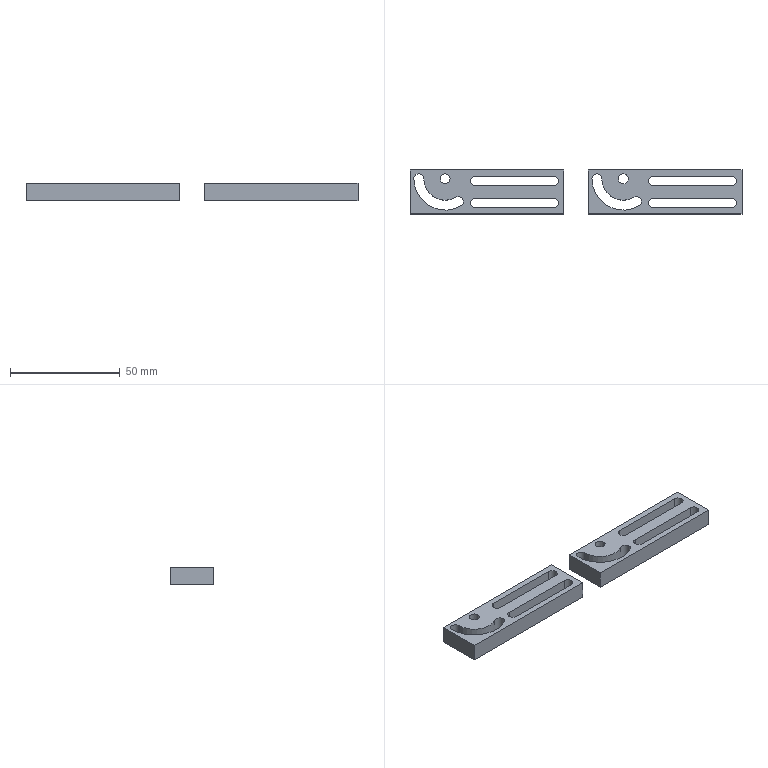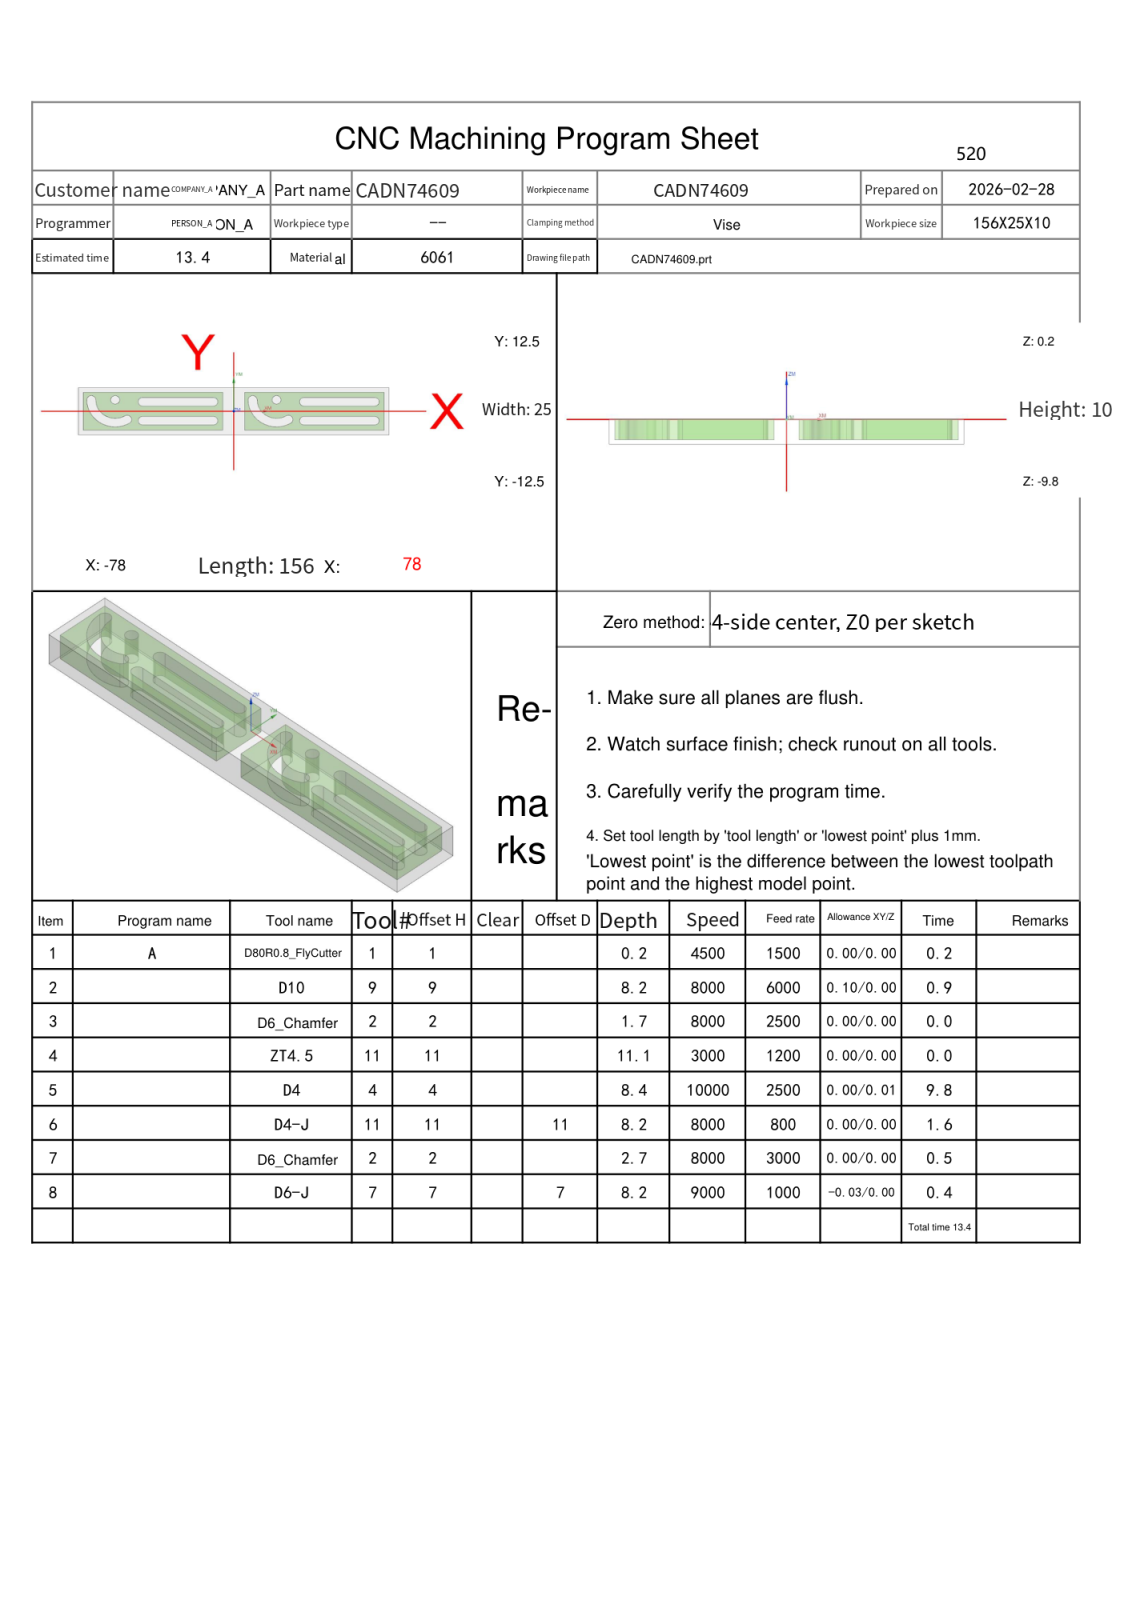NC program | NX | posted by the shop | part box 151 x 20 x 8 mm
Lines 276 to 1289 of 3746:
N5 T04 M06
(D4  D=4. R=0. H=04 ce=0.10 di=0.10)
G00 G90 G54 X-28. Y4.85 M03 S10000
G43 H04 Z50.
M08
Z.5
G01 X-10.25 Z.439 F1200.
G03 X-10.1 Y5. Z.438 I0.0 J.15
X-10.25 Y5.15 Z.437 I-.15 J0.0
G01 X-45.75 Z.314
G03 X-45.9 Y5. Z.314 I0.0 J-.15
X-45.75 Y4.85 Z.313 I.15 J0.0
G01 X-10.25 Z.19
G03 X-10.1 Y5. Z.189 I0.0 J.15
X-10.25 Y5.15 Z.188 I-.15 J0.0
G01 X-45.75 Z.066
G03 X-45.9 Y5. Z.065 I0.0 J-.15
X-45.75 Y4.85 Z.064 I.15 J0.0
G01 X-10.25 Z-.058
G03 X-10.1 Y5. Z-.059 I0.0 J.15
X-10.25 Y5.15 Z-.06 I-.15 J0.0
G01 X-45.75 Z-.183
G03 X-45.9 Y5. Z-.184 I0.0 J-.15
X-45.75 Y4.85 Z-.184 I.15 J0.0
G01 X-10.25 Z-.307
G03 X-10.1 Y5. Z-.308 I0.0 J.15
X-10.25 Y5.15 Z-.309 I-.15 J0.0
G01 X-45.75 Z-.431
G03 X-45.9 Y5. Z-.432 I0.0 J-.15
X-45.75 Y4.85 Z-.433 I.15 J0.0
G01 X-10.25 Z-.556
G03 X-10.1 Y5. Z-.556 I0.0 J.15
X-10.25 Y5.15 Z-.557 I-.15 J0.0
G01 X-45.75 Z-.68
G03 X-45.9 Y5. Z-.681 I0.0 J-.15
X-45.75 Y4.85 Z-.682 I.15 J0.0
G01 X-10.25 Z-.804
G03 X-10.1 Y5. Z-.805 I0.0 J.15
X-10.25 Y5.15 Z-.806 I-.15 J0.0
G01 X-45.75 Z-.928
G03 X-45.9 Y5. Z-.929 I0.0 J-.15
X-45.75 Y4.85 Z-.93 I.15 J0.0
G01 X-10.25 Z-1.053
G03 X-10.1 Y5. Z-1.054 I0.0 J.15
X-10.25 Y5.15 Z-1.054 I-.15 J0.0
G01 X-45.75 Z-1.177
G03 X-45.9 Y5. Z-1.178 I0.0 J-.15
X-45.75 Y4.85 Z-1.179 I.15 J0.0
G01 X-10.25 Z-1.301
G03 X-10.1 Y5. Z-1.302 I0.0 J.15
X-10.25 Y5.15 Z-1.303 I-.15 J0.0
G01 X-45.75 Z-1.426
G03 X-45.9 Y5. Z-1.426 I0.0 J-.15
X-45.75 Y4.85 Z-1.427 I.15 J0.0
G01 X-10.25 Z-1.55
G03 X-10.1 Y5. Z-1.551 I0.0 J.15
X-10.25 Y5.15 Z-1.552 I-.15 J0.0
G01 X-45.75 Z-1.674
G03 X-45.9 Y5. Z-1.675 I0.0 J-.15
X-45.75 Y4.85 Z-1.676 I.15 J0.0
G01 X-10.25 Z-1.798
G03 X-10.1 Y5. Z-1.799 I0.0 J.15
X-10.25 Y5.15 Z-1.8 I-.15 J0.0
G01 X-45.75 Z-1.923
G03 X-45.9 Y5. Z-1.924 I0.0 J-.15
X-45.75 Y4.85 Z-1.924 I.15 J0.0
G01 X-10.25 Z-2.047
G03 X-10.1 Y5. Z-2.048 I0.0 J.15
X-10.25 Y5.15 Z-2.049 I-.15 J0.0
G01 X-45.75 Z-2.171
G03 X-45.9 Y5. Z-2.172 I0.0 J-.15
X-45.75 Y4.85 Z-2.173 I.15 J0.0
G01 X-10.25 Z-2.296
G03 X-10.1 Y5. Z-2.296 I0.0 J.15
X-10.25 Y5.15 Z-2.297 I-.15 J0.0
G01 X-45.75 Z-2.42
G03 X-45.9 Y5. Z-2.421 I0.0 J-.15
X-45.75 Y4.85 Z-2.422 I.15 J0.0
G01 X-10.25 Z-2.544
G03 X-10.1 Y5. Z-2.545 I0.0 J.15
X-10.25 Y5.15 Z-2.546 I-.15 J0.0
G01 X-45.75 Z-2.668
G03 X-45.9 Y5. Z-2.669 I0.0 J-.15
X-45.75 Y4.85 Z-2.67 I.15 J0.0
G01 X-10.25 Z-2.793
G03 X-10.1 Y5. Z-2.794 I0.0 J.15
X-10.25 Y5.15 Z-2.794 I-.15 J0.0
G01 X-45.75 Z-2.917
G03 X-45.9 Y5. Z-2.918 I0.0 J-.15
X-45.75 Y4.85 Z-2.919 I.15 J0.0
G01 X-10.25 Z-3.041
G03 X-10.1 Y5. Z-3.042 I0.0 J.15
X-10.25 Y5.15 Z-3.043 I-.15 J0.0
G01 X-45.75 Z-3.166
G03 X-45.9 Y5. Z-3.166 I0.0 J-.15
X-45.75 Y4.85 Z-3.167 I.15 J0.0
G01 X-10.25 Z-3.29
G03 X-10.1 Y5. Z-3.291 I0.0 J.15
X-10.25 Y5.15 Z-3.292 I-.15 J0.0
G01 X-45.75 Z-3.414
G03 X-45.9 Y5. Z-3.415 I0.0 J-.15
X-45.75 Y4.85 Z-3.416 I.15 J0.0
G01 X-10.25 Z-3.538
G03 X-10.1 Y5. Z-3.539 I0.0 J.15
X-10.25 Y5.15 Z-3.54 I-.15 J0.0
G01 X-45.75 Z-3.663
G03 X-45.9 Y5. Z-3.664 I0.0 J-.15
X-45.75 Y4.85 Z-3.664 I.15 J0.0
G01 X-10.25 Z-3.787
G03 X-10.1 Y5. Z-3.788 I0.0 J.15
X-10.25 Y5.15 Z-3.789 I-.15 J0.0
G01 X-45.75 Z-3.911
G03 X-45.9 Y5. Z-3.912 I0.0 J-.15
X-45.75 Y4.85 Z-3.913 I.15 J0.0
G01 X-10.25 Z-4.036
G03 X-10.1 Y5. Z-4.036 I0.0 J.15
X-10.25 Y5.15 Z-4.037 I-.15 J0.0
G01 X-45.75 Z-4.16
G03 X-45.9 Y5. Z-4.161 I0.0 J-.15
X-45.75 Y4.85 Z-4.162 I.15 J0.0
G01 X-10.25 Z-4.284
G03 X-10.1 Y5. Z-4.285 I0.0 J.15
X-10.25 Y5.15 Z-4.286 I-.15 J0.0
G01 X-45.75 Z-4.408
G03 X-45.9 Y5. Z-4.409 I0.0 J-.15
X-45.75 Y4.85 Z-4.41 I.15 J0.0
G01 X-10.25 Z-4.533
G03 X-10.1 Y5. Z-4.534 I0.0 J.15
X-10.25 Y5.15 Z-4.534 I-.15 J0.0
G01 X-45.75 Z-4.657
G03 X-45.9 Y5. Z-4.658 I0.0 J-.15
X-45.75 Y4.85 Z-4.659 I.15 J0.0
G01 X-10.25 Z-4.781
G03 X-10.1 Y5. Z-4.782 I0.0 J.15
X-10.25 Y5.15 Z-4.783 I-.15 J0.0
G01 X-45.75 Z-4.906
G03 X-45.9 Y5. Z-4.906 I0.0 J-.15
X-45.75 Y4.85 Z-4.907 I.15 J0.0
G01 X-10.25 Z-5.03
G03 X-10.1 Y5. Z-5.031 I0.0 J.15
X-10.25 Y5.15 Z-5.032 I-.15 J0.0
G01 X-45.75 Z-5.154
G03 X-45.9 Y5. Z-5.155 I0.0 J-.15
X-45.75 Y4.85 Z-5.156 I.15 J0.0
G01 X-10.25 Z-5.278
G03 X-10.1 Y5. Z-5.279 I0.0 J.15
X-10.25 Y5.15 Z-5.28 I-.15 J0.0
G01 X-45.75 Z-5.403
G03 X-45.9 Y5. Z-5.404 I0.0 J-.15
X-45.75 Y4.85 Z-5.404 I.15 J0.0
G01 X-10.25 Z-5.527
G03 X-10.1 Y5. Z-5.528 I0.0 J.15
X-10.25 Y5.15 Z-5.529 I-.15 J0.0
G01 X-45.75 Z-5.651
G03 X-45.9 Y5. Z-5.652 I0.0 J-.15
X-45.75 Y4.85 Z-5.653 I.15 J0.0
G01 X-10.25 Z-5.776
G03 X-10.1 Y5. Z-5.776 I0.0 J.15
X-10.25 Y5.15 Z-5.777 I-.15 J0.0
G01 X-45.75 Z-5.9
G03 X-45.9 Y5. Z-5.901 I0.0 J-.15
X-45.75 Y4.85 Z-5.902 I.15 J0.0
G01 X-10.25 Z-6.024
G03 X-10.1 Y5. Z-6.025 I0.0 J.15
X-10.25 Y5.15 Z-6.026 I-.15 J0.0
G01 X-45.75 Z-6.148
G03 X-45.9 Y5. Z-6.149 I0.0 J-.15
X-45.75 Y4.85 Z-6.15 I.15 J0.0
G01 X-10.25 Z-6.273
G03 X-10.1 Y5. Z-6.274 I0.0 J.15
X-10.25 Y5.15 Z-6.274 I-.15 J0.0
G01 X-45.75 Z-6.397
G03 X-45.9 Y5. Z-6.398 I0.0 J-.15
X-45.75 Y4.85 Z-6.399 I.15 J0.0
G01 X-10.25 Z-6.521
G03 X-10.1 Y5. Z-6.522 I0.0 J.15
X-10.25 Y5.15 Z-6.523 I-.15 J0.0
G01 X-45.75 Z-6.646
G03 X-45.9 Y5. Z-6.646 I0.0 J-.15
X-45.75 Y4.85 Z-6.647 I.15 J0.0
G01 X-10.25 Z-6.77
G03 X-10.1 Y5. Z-6.771 I0.0 J.15
X-10.25 Y5.15 Z-6.772 I-.15 J0.0
G01 X-45.75 Z-6.894
G03 X-45.9 Y5. Z-6.895 I0.0 J-.15
X-45.75 Y4.85 Z-6.896 I.15 J0.0
G01 X-10.25 Z-7.018
G03 X-10.1 Y5. Z-7.019 I0.0 J.15
X-10.25 Y5.15 Z-7.02 I-.15 J0.0
G01 X-45.75 Z-7.143
G03 X-45.9 Y5. Z-7.144 I0.0 J-.15
X-45.75 Y4.85 Z-7.144 I.15 J0.0
G01 X-10.25 Z-7.267
G03 X-10.1 Y5. Z-7.268 I0.0 J.15
X-10.25 Y5.15 Z-7.269 I-.15 J0.0
G01 X-45.75 Z-7.391
G03 X-45.9 Y5. Z-7.392 I0.0 J-.15
X-45.75 Y4.85 Z-7.393 I.15 J0.0
G01 X-10.25 Z-7.516
G03 X-10.1 Y5. Z-7.516 I0.0 J.15
X-10.25 Y5.15 Z-7.517 I-.15 J0.0
G01 X-45.75 Z-7.64
G03 X-45.9 Y5. Z-7.641 I0.0 J-.15
X-45.75 Y4.85 Z-7.642 I.15 J0.0
G01 X-10.25 Z-7.764
G03 X-10.1 Y5. Z-7.765 I0.0 J.15
X-10.25 Y5.15 Z-7.766 I-.15 J0.0
G01 X-45.75 Z-7.888
G03 X-45.9 Y5. Z-7.889 I0.0 J-.15
X-45.75 Y4.85 Z-7.89 I.15 J0.0
G01 X-10.25 Z-8.013
G03 X-10.1 Y5. Z-8.014 I0.0 J.15
X-10.25 Y5.15 Z-8.014 I-.15 J0.0
G01 X-45.75 Z-8.137
G03 X-45.9 Y5. Z-8.138 I0.0 J-.15
X-45.75 Y4.85 Z-8.139 I.15 J0.0
G01 X-28. Z-8.2
X-10.25
G03 X-10.1 Y5. I0.0 J.15
X-10.25 Y5.15 I-.15 J0.0
G01 X-45.75
G03 X-45.9 Y5. I0.0 J-.15
X-45.75 Y4.85 I.15 J0.0
G01 X-28.
X-27.5
Z-7.2
G00 Z50.
X-28. Y-4.85
Z.5
G01 X-45.75 Z.439
G03 X-45.9 Y-5. Z.438 I0.0 J-.15
X-45.75 Y-5.15 Z.437 I.15 J0.0
G01 X-10.25 Z.314
G03 X-10.1 Y-5. Z.314 I0.0 J.15
X-10.25 Y-4.85 Z.313 I-.15 J0.0
G01 X-45.75 Z.19
G03 X-45.9 Y-5. Z.189 I0.0 J-.15
X-45.75 Y-5.15 Z.188 I.15 J0.0
G01 X-10.25 Z.066
G03 X-10.1 Y-5. Z.065 I0.0 J.15
X-10.25 Y-4.85 Z.064 I-.15 J0.0
G01 X-45.75 Z-.058
G03 X-45.9 Y-5. Z-.059 I0.0 J-.15
X-45.75 Y-5.15 Z-.06 I.15 J0.0
G01 X-10.25 Z-.183
G03 X-10.1 Y-5. Z-.184 I0.0 J.15
X-10.25 Y-4.85 Z-.184 I-.15 J0.0
G01 X-45.75 Z-.307
G03 X-45.9 Y-5. Z-.308 I0.0 J-.15
X-45.75 Y-5.15 Z-.309 I.15 J0.0
G01 X-10.25 Z-.431
G03 X-10.1 Y-5. Z-.432 I0.0 J.15
X-10.25 Y-4.85 Z-.433 I-.15 J0.0
G01 X-45.75 Z-.556
G03 X-45.9 Y-5. Z-.556 I0.0 J-.15
X-45.75 Y-5.15 Z-.557 I.15 J0.0
G01 X-10.25 Z-.68
G03 X-10.1 Y-5. Z-.681 I0.0 J.15
X-10.25 Y-4.85 Z-.682 I-.15 J0.0
G01 X-45.75 Z-.804
G03 X-45.9 Y-5. Z-.805 I0.0 J-.15
X-45.75 Y-5.15 Z-.806 I.15 J0.0
G01 X-10.25 Z-.928
G03 X-10.1 Y-5. Z-.929 I0.0 J.15
X-10.25 Y-4.85 Z-.93 I-.15 J0.0
G01 X-45.75 Z-1.053
G03 X-45.9 Y-5. Z-1.054 I0.0 J-.15
X-45.75 Y-5.15 Z-1.054 I.15 J0.0
G01 X-10.25 Z-1.177
G03 X-10.1 Y-5. Z-1.178 I0.0 J.15
X-10.25 Y-4.85 Z-1.179 I-.15 J0.0
G01 X-45.75 Z-1.301
G03 X-45.9 Y-5. Z-1.302 I0.0 J-.15
X-45.75 Y-5.15 Z-1.303 I.15 J0.0
G01 X-10.25 Z-1.426
G03 X-10.1 Y-5. Z-1.426 I0.0 J.15
X-10.25 Y-4.85 Z-1.427 I-.15 J0.0
G01 X-45.75 Z-1.55
G03 X-45.9 Y-5. Z-1.551 I0.0 J-.15
X-45.75 Y-5.15 Z-1.552 I.15 J0.0
G01 X-10.25 Z-1.674
G03 X-10.1 Y-5. Z-1.675 I0.0 J.15
X-10.25 Y-4.85 Z-1.676 I-.15 J0.0
G01 X-45.75 Z-1.798
G03 X-45.9 Y-5. Z-1.799 I0.0 J-.15
X-45.75 Y-5.15 Z-1.8 I.15 J0.0
G01 X-10.25 Z-1.923
G03 X-10.1 Y-5. Z-1.924 I0.0 J.15
X-10.25 Y-4.85 Z-1.924 I-.15 J0.0
G01 X-45.75 Z-2.047
G03 X-45.9 Y-5. Z-2.048 I0.0 J-.15
X-45.75 Y-5.15 Z-2.049 I.15 J0.0
G01 X-10.25 Z-2.171
G03 X-10.1 Y-5. Z-2.172 I0.0 J.15
X-10.25 Y-4.85 Z-2.173 I-.15 J0.0
G01 X-45.75 Z-2.296
G03 X-45.9 Y-5. Z-2.296 I0.0 J-.15
X-45.75 Y-5.15 Z-2.297 I.15 J0.0
G01 X-10.25 Z-2.42
G03 X-10.1 Y-5. Z-2.421 I0.0 J.15
X-10.25 Y-4.85 Z-2.422 I-.15 J0.0
G01 X-45.75 Z-2.544
G03 X-45.9 Y-5. Z-2.545 I0.0 J-.15
X-45.75 Y-5.15 Z-2.546 I.15 J0.0
G01 X-10.25 Z-2.668
G03 X-10.1 Y-5. Z-2.669 I0.0 J.15
X-10.25 Y-4.85 Z-2.67 I-.15 J0.0
G01 X-45.75 Z-2.793
G03 X-45.9 Y-5. Z-2.794 I0.0 J-.15
X-45.75 Y-5.15 Z-2.794 I.15 J0.0
G01 X-10.25 Z-2.917
G03 X-10.1 Y-5. Z-2.918 I0.0 J.15
X-10.25 Y-4.85 Z-2.919 I-.15 J0.0
G01 X-45.75 Z-3.041
G03 X-45.9 Y-5. Z-3.042 I0.0 J-.15
X-45.75 Y-5.15 Z-3.043 I.15 J0.0
G01 X-10.25 Z-3.166
G03 X-10.1 Y-5. Z-3.166 I0.0 J.15
X-10.25 Y-4.85 Z-3.167 I-.15 J0.0
G01 X-45.75 Z-3.29
G03 X-45.9 Y-5. Z-3.291 I0.0 J-.15
X-45.75 Y-5.15 Z-3.292 I.15 J0.0
G01 X-10.25 Z-3.414
G03 X-10.1 Y-5. Z-3.415 I0.0 J.15
X-10.25 Y-4.85 Z-3.416 I-.15 J0.0
G01 X-45.75 Z-3.538
G03 X-45.9 Y-5. Z-3.539 I0.0 J-.15
X-45.75 Y-5.15 Z-3.54 I.15 J0.0
G01 X-10.25 Z-3.663
G03 X-10.1 Y-5. Z-3.664 I0.0 J.15
X-10.25 Y-4.85 Z-3.664 I-.15 J0.0
G01 X-45.75 Z-3.787
G03 X-45.9 Y-5. Z-3.788 I0.0 J-.15
X-45.75 Y-5.15 Z-3.789 I.15 J0.0
G01 X-10.25 Z-3.911
G03 X-10.1 Y-5. Z-3.912 I0.0 J.15
X-10.25 Y-4.85 Z-3.913 I-.15 J0.0
G01 X-45.75 Z-4.036
G03 X-45.9 Y-5. Z-4.036 I0.0 J-.15
X-45.75 Y-5.15 Z-4.037 I.15 J0.0
G01 X-10.25 Z-4.16
G03 X-10.1 Y-5. Z-4.161 I0.0 J.15
X-10.25 Y-4.85 Z-4.162 I-.15 J0.0
G01 X-45.75 Z-4.284
G03 X-45.9 Y-5. Z-4.285 I0.0 J-.15
X-45.75 Y-5.15 Z-4.286 I.15 J0.0
G01 X-10.25 Z-4.408
G03 X-10.1 Y-5. Z-4.409 I0.0 J.15
X-10.25 Y-4.85 Z-4.41 I-.15 J0.0
G01 X-45.75 Z-4.533
G03 X-45.9 Y-5. Z-4.534 I0.0 J-.15
X-45.75 Y-5.15 Z-4.534 I.15 J0.0
G01 X-10.25 Z-4.657
G03 X-10.1 Y-5. Z-4.658 I0.0 J.15
X-10.25 Y-4.85 Z-4.659 I-.15 J0.0
G01 X-45.75 Z-4.781
G03 X-45.9 Y-5. Z-4.782 I0.0 J-.15
X-45.75 Y-5.15 Z-4.783 I.15 J0.0
G01 X-10.25 Z-4.906
G03 X-10.1 Y-5. Z-4.906 I0.0 J.15
X-10.25 Y-4.85 Z-4.907 I-.15 J0.0
G01 X-45.75 Z-5.03
G03 X-45.9 Y-5. Z-5.031 I0.0 J-.15
X-45.75 Y-5.15 Z-5.032 I.15 J0.0
G01 X-10.25 Z-5.154
G03 X-10.1 Y-5. Z-5.155 I0.0 J.15
X-10.25 Y-4.85 Z-5.156 I-.15 J0.0
G01 X-45.75 Z-5.278
G03 X-45.9 Y-5. Z-5.279 I0.0 J-.15
X-45.75 Y-5.15 Z-5.28 I.15 J0.0
G01 X-10.25 Z-5.403
G03 X-10.1 Y-5. Z-5.404 I0.0 J.15
X-10.25 Y-4.85 Z-5.404 I-.15 J0.0
G01 X-45.75 Z-5.527
G03 X-45.9 Y-5. Z-5.528 I0.0 J-.15
X-45.75 Y-5.15 Z-5.529 I.15 J0.0
G01 X-10.25 Z-5.651
G03 X-10.1 Y-5. Z-5.652 I0.0 J.15
X-10.25 Y-4.85 Z-5.653 I-.15 J0.0
G01 X-45.75 Z-5.776
G03 X-45.9 Y-5. Z-5.776 I0.0 J-.15
X-45.75 Y-5.15 Z-5.777 I.15 J0.0
G01 X-10.25 Z-5.9
G03 X-10.1 Y-5. Z-5.901 I0.0 J.15
X-10.25 Y-4.85 Z-5.902 I-.15 J0.0
G01 X-45.75 Z-6.024
G03 X-45.9 Y-5. Z-6.025 I0.0 J-.15
X-45.75 Y-5.15 Z-6.026 I.15 J0.0
G01 X-10.25 Z-6.148
G03 X-10.1 Y-5. Z-6.149 I0.0 J.15
X-10.25 Y-4.85 Z-6.15 I-.15 J0.0
G01 X-45.75 Z-6.273
G03 X-45.9 Y-5. Z-6.274 I0.0 J-.15
X-45.75 Y-5.15 Z-6.274 I.15 J0.0
G01 X-10.25 Z-6.397
G03 X-10.1 Y-5. Z-6.398 I0.0 J.15
X-10.25 Y-4.85 Z-6.399 I-.15 J0.0
G01 X-45.75 Z-6.521
G03 X-45.9 Y-5. Z-6.522 I0.0 J-.15
X-45.75 Y-5.15 Z-6.523 I.15 J0.0
G01 X-10.25 Z-6.646
G03 X-10.1 Y-5. Z-6.646 I0.0 J.15
X-10.25 Y-4.85 Z-6.647 I-.15 J0.0
G01 X-45.75 Z-6.77
G03 X-45.9 Y-5. Z-6.771 I0.0 J-.15
X-45.75 Y-5.15 Z-6.772 I.15 J0.0
G01 X-10.25 Z-6.894
G03 X-10.1 Y-5. Z-6.895 I0.0 J.15
X-10.25 Y-4.85 Z-6.896 I-.15 J0.0
G01 X-45.75 Z-7.018
G03 X-45.9 Y-5. Z-7.019 I0.0 J-.15
X-45.75 Y-5.15 Z-7.02 I.15 J0.0
G01 X-10.25 Z-7.143
G03 X-10.1 Y-5. Z-7.144 I0.0 J.15
X-10.25 Y-4.85 Z-7.144 I-.15 J0.0
G01 X-45.75 Z-7.267
G03 X-45.9 Y-5. Z-7.268 I0.0 J-.15
X-45.75 Y-5.15 Z-7.269 I.15 J0.0
G01 X-10.25 Z-7.391
G03 X-10.1 Y-5. Z-7.392 I0.0 J.15
X-10.25 Y-4.85 Z-7.393 I-.15 J0.0
G01 X-45.75 Z-7.516
G03 X-45.9 Y-5. Z-7.516 I0.0 J-.15
X-45.75 Y-5.15 Z-7.517 I.15 J0.0
G01 X-10.25 Z-7.64
G03 X-10.1 Y-5. Z-7.641 I0.0 J.15
X-10.25 Y-4.85 Z-7.642 I-.15 J0.0
G01 X-45.75 Z-7.764
G03 X-45.9 Y-5. Z-7.765 I0.0 J-.15
X-45.75 Y-5.15 Z-7.766 I.15 J0.0
G01 X-10.25 Z-7.888
G03 X-10.1 Y-5. Z-7.889 I0.0 J.15
X-10.25 Y-4.85 Z-7.89 I-.15 J0.0
G01 X-45.75 Z-8.013
G03 X-45.9 Y-5. Z-8.014 I0.0 J-.15
X-45.75 Y-5.15 Z-8.014 I.15 J0.0
G01 X-10.25 Z-8.137
G03 X-10.1 Y-5. Z-8.138 I0.0 J.15
X-10.25 Y-4.85 Z-8.139 I-.15 J0.0
G01 X-28. Z-8.2
X-45.75
G03 X-45.9 Y-5. I0.0 J-.15
X-45.75 Y-5.15 I.15 J0.0
G01 X-10.25
G03 X-10.1 Y-5. I0.0 J.15
X-10.25 Y-4.85 I-.15 J0.0
G01 X-28.
X-28.5
Z-7.2
G00 Z50.
X53. Y4.85
Z.5
G01 X70.75 Z.439
X70.807 Z.438
X70.856 Y4.88
X70.883 Y4.93
X70.905 Y4.962
X70.9 Y5.
G03 X70.75 Y5.15 Z.437 I-.15 J0.0
G01 X35.25 Z.314
G03 X35.1 Y5. Z.314 I0.0 J-.15
X35.25 Y4.85 Z.313 I.15 J0.0
G01 X70.75 Z.19
X70.807
X70.856 Y4.88
X70.883 Y4.93
X70.905 Y4.962 Z.189
X70.9 Y5.
G03 X70.75 Y5.15 Z.188 I-.15 J0.0
G01 X35.25 Z.066
G03 X35.1 Y5. Z.065 I0.0 J-.15
X35.25 Y4.85 Z.064 I.15 J0.0
G01 X70.75 Z-.058
X70.807 Z-.059
X70.856 Y4.88
X70.883 Y4.93
X70.905 Y4.962
X70.9 Y5.
G03 X70.75 Y5.15 Z-.06 I-.15 J0.0
G01 X35.25 Z-.183
G03 X35.1 Y5. Z-.184 I0.0 J-.15
X35.25 Y4.85 Z-.184 I.15 J0.0
G01 X70.75 Z-.307
X70.807
X70.856 Y4.88
X70.883 Y4.93 Z-.308
X70.905 Y4.962
X70.9 Y5.
G03 X70.75 Y5.15 Z-.309 I-.15 J0.0
G01 X35.25 Z-.431
G03 X35.1 Y5. Z-.432 I0.0 J-.15
X35.25 Y4.85 Z-.433 I.15 J0.0
G01 X70.75 Z-.556
X70.807
X70.856 Y4.88
X70.883 Y4.93
X70.905 Y4.962
X70.9 Y5.
G03 X70.75 Y5.15 Z-.557 I-.15 J0.0
G01 X35.25 Z-.68
G03 X35.1 Y5. Z-.681 I0.0 J-.15
X35.25 Y4.85 Z-.682 I.15 J0.0
G01 X70.75 Z-.804
X70.807
X70.856 Y4.88 Z-.805
X70.883 Y4.93
X70.905 Y4.962
X70.9 Y5.
G03 X70.75 Y5.15 Z-.806 I-.15 J0.0
G01 X35.25 Z-.928
G03 X35.1 Y5. Z-.929 I0.0 J-.15
X35.25 Y4.85 Z-.93 I.15 J0.0
G01 X70.75 Z-1.053
X70.807
X70.856 Y4.88
X70.883 Y4.93
X70.905 Y4.962
X70.9 Y5. Z-1.054
G03 X70.75 Y5.15 Z-1.054 I-.15 J0.0
G01 X35.25 Z-1.177
G03 X35.1 Y5. Z-1.178 I0.0 J-.15
X35.25 Y4.85 Z-1.179 I.15 J0.0
G01 X70.75 Z-1.301
X70.807 Z-1.302
X70.856 Y4.88
X70.883 Y4.93
X70.905 Y4.962
X70.9 Y5.
G03 X70.75 Y5.15 Z-1.303 I-.15 J0.0
G01 X35.25 Z-1.426
G03 X35.1 Y5. Z-1.426 I0.0 J-.15
X35.25 Y4.85 Z-1.427 I.15 J0.0
G01 X70.75 Z-1.55
X70.807
X70.856 Y4.88
X70.883 Y4.93
X70.905 Y4.962 Z-1.551
X70.9 Y5.
G03 X70.75 Y5.15 Z-1.552 I-.15 J0.0
G01 X35.25 Z-1.674
G03 X35.1 Y5. Z-1.675 I0.0 J-.15
X35.25 Y4.85 Z-1.676 I.15 J0.0
G01 X70.75 Z-1.798
X70.807 Z-1.799
X70.856 Y4.88
X70.883 Y4.93
X70.905 Y4.962
X70.9 Y5.
G03 X70.75 Y5.15 Z-1.8 I-.15 J0.0
G01 X35.25 Z-1.923
G03 X35.1 Y5. Z-1.924 I0.0 J-.15
X35.25 Y4.85 Z-1.924 I.15 J0.0
G01 X70.75 Z-2.047
X70.807
X70.856 Y4.88
X70.883 Y4.93 Z-2.048
X70.905 Y4.962
X70.9 Y5.
G03 X70.75 Y5.15 Z-2.049 I-.15 J0.0
G01 X35.25 Z-2.171
G03 X35.1 Y5. Z-2.172 I0.0 J-.15
X35.25 Y4.85 Z-2.173 I.15 J0.0
G01 X70.75 Z-2.296
X70.807
X70.856 Y4.88
X70.883 Y4.93
X70.905 Y4.962
X70.9 Y5.
G03 X70.75 Y5.15 Z-2.297 I-.15 J0.0
G01 X35.25 Z-2.42
G03 X35.1 Y5. Z-2.421 I0.0 J-.15
X35.25 Y4.85 Z-2.422 I.15 J0.0
G01 X70.75 Z-2.544
X70.807
X70.856 Y4.88 Z-2.545
X70.883 Y4.93
X70.905 Y4.962
X70.9 Y5.
G03 X70.75 Y5.15 Z-2.546 I-.15 J0.0
G01 X35.25 Z-2.668
G03 X35.1 Y5. Z-2.669 I0.0 J-.15
X35.25 Y4.85 Z-2.67 I.15 J0.0
G01 X70.75 Z-2.793
X70.807
X70.856 Y4.88
X70.883 Y4.93
X70.905 Y4.962
X70.9 Y5. Z-2.794
G03 X70.75 Y5.15 Z-2.794 I-.15 J0.0
G01 X35.25 Z-2.917
G03 X35.1 Y5. Z-2.918 I0.0 J-.15
X35.25 Y4.85 Z-2.919 I.15 J0.0
G01 X70.75 Z-3.041
X70.807 Z-3.042
X70.856 Y4.88
X70.883 Y4.93
X70.905 Y4.962
X70.9 Y5.
G03 X70.75 Y5.15 Z-3.043 I-.15 J0.0
G01 X35.25 Z-3.166
G03 X35.1 Y5. Z-3.166 I0.0 J-.15
X35.25 Y4.85 Z-3.167 I.15 J0.0
G01 X70.75 Z-3.29
X70.807
X70.856 Y4.88
X70.883 Y4.93
X70.905 Y4.962 Z-3.291
X70.9 Y5.
G03 X70.75 Y5.15 Z-3.292 I-.15 J0.0
G01 X35.25 Z-3.414
G03 X35.1 Y5. Z-3.415 I0.0 J-.15
X35.25 Y4.85 Z-3.416 I.15 J0.0
G01 X70.75 Z-3.538
X70.807 Z-3.539
X70.856 Y4.88
X70.883 Y4.93
X70.905 Y4.962
X70.9 Y5.
G03 X70.75 Y5.15 Z-3.54 I-.15 J0.0
G01 X35.25 Z-3.663
G03 X35.1 Y5. Z-3.664 I0.0 J-.15
X35.25 Y4.85 Z-3.664 I.15 J0.0
G01 X70.75 Z-3.787
X70.807
X70.856 Y4.88
X70.883 Y4.93 Z-3.788
X70.905 Y4.962
X70.9 Y5.
G03 X70.75 Y5.15 Z-3.789 I-.15 J0.0
G01 X35.25 Z-3.911
G03 X35.1 Y5. Z-3.912 I0.0 J-.15
X35.25 Y4.85 Z-3.913 I.15 J0.0
G01 X70.75 Z-4.036
X70.807
X70.856 Y4.88
X70.883 Y4.93
X70.905 Y4.962
X70.9 Y5.
G03 X70.75 Y5.15 Z-4.037 I-.15 J0.0
G01 X35.25 Z-4.16
G03 X35.1 Y5. Z-4.161 I0.0 J-.15
X35.25 Y4.85 Z-4.162 I.15 J0.0
G01 X70.75 Z-4.284
X70.807
X70.856 Y4.88 Z-4.285
X70.883 Y4.93
X70.905 Y4.962
X70.9 Y5.
G03 X70.75 Y5.15 Z-4.286 I-.15 J0.0
G01 X35.25 Z-4.408
G03 X35.1 Y5. Z-4.409 I0.0 J-.15
X35.25 Y4.85 Z-4.41 I.15 J0.0
G01 X70.75 Z-4.533
X70.807
X70.856 Y4.88
X70.883 Y4.93
X70.905 Y4.962
X70.9 Y5. Z-4.534
G03 X70.75 Y5.15 Z-4.534 I-.15 J0.0
G01 X35.25 Z-4.657
G03 X35.1 Y5. Z-4.658 I0.0 J-.15
X35.25 Y4.85 Z-4.659 I.15 J0.0
G01 X70.75 Z-4.781
X70.807 Z-4.782
X70.856 Y4.88
X70.883 Y4.93
X70.905 Y4.962
X70.9 Y5.
G03 X70.75 Y5.15 Z-4.783 I-.15 J0.0
G01 X35.25 Z-4.906
G03 X35.1 Y5. Z-4.906 I0.0 J-.15
X35.25 Y4.85 Z-4.907 I.15 J0.0
G01 X70.75 Z-5.03
X70.807
X70.856 Y4.88
X70.883 Y4.93
X70.905 Y4.962 Z-5.031
X70.9 Y5.
G03 X70.75 Y5.15 Z-5.032 I-.15 J0.0
G01 X35.25 Z-5.154
G03 X35.1 Y5. Z-5.155 I0.0 J-.15
X35.25 Y4.85 Z-5.156 I.15 J0.0
G01 X70.75 Z-5.278
X70.807 Z-5.279
X70.856 Y4.88
X70.883 Y4.93
X70.905 Y4.962
X70.9 Y5.
G03 X70.75 Y5.15 Z-5.28 I-.15 J0.0
G01 X35.25 Z-5.403
G03 X35.1 Y5. Z-5.404 I0.0 J-.15
X35.25 Y4.85 Z-5.404 I.15 J0.0
G01 X70.75 Z-5.527
X70.807
X70.856 Y4.88
X70.883 Y4.93 Z-5.528
X70.905 Y4.962
X70.9 Y5.
G03 X70.75 Y5.15 Z-5.529 I-.15 J0.0
G01 X35.25 Z-5.651
G03 X35.1 Y5. Z-5.652 I0.0 J-.15
X35.25 Y4.85 Z-5.653 I.15 J0.0
G01 X70.75 Z-5.776
X70.807
X70.856 Y4.88
X70.883 Y4.93
X70.905 Y4.962
X70.9 Y5.
G03 X70.75 Y5.15 Z-5.777 I-.15 J0.0
G01 X35.25 Z-5.9
G03 X35.1 Y5. Z-5.901 I0.0 J-.15
X35.25 Y4.85 Z-5.902 I.15 J0.0
G01 X70.75 Z-6.024
X70.807
X70.856 Y4.88 Z-6.025
X70.883 Y4.93
X70.905 Y4.962
X70.9 Y5.
G03 X70.75 Y5.15 Z-6.026 I-.15 J0.0
G01 X35.25 Z-6.148
G03 X35.1 Y5. Z-6.149 I0.0 J-.15
X35.25 Y4.85 Z-6.15 I.15 J0.0
G01 X70.75 Z-6.273
X70.807
X70.856 Y4.88
X70.883 Y4.93
X70.905 Y4.962
X70.9 Y5. Z-6.274
G03 X70.75 Y5.15 Z-6.274 I-.15 J0.0
G01 X35.25 Z-6.397
G03 X35.1 Y5. Z-6.398 I0.0 J-.15
X35.25 Y4.85 Z-6.399 I.15 J0.0
G01 X70.75 Z-6.521
X70.807 Z-6.522
X70.856 Y4.88
X70.883 Y4.93
X70.905 Y4.962
X70.9 Y5.
G03 X70.75 Y5.15 Z-6.523 I-.15 J0.0
G01 X35.25 Z-6.646
G03 X35.1 Y5. Z-6.646 I0.0 J-.15
X35.25 Y4.85 Z-6.647 I.15 J0.0
G01 X70.75 Z-6.77
X70.807
X70.856 Y4.88
X70.883 Y4.93
X70.905 Y4.962 Z-6.771
X70.9 Y5.
G03 X70.75 Y5.15 Z-6.772 I-.15 J0.0
G01 X35.25 Z-6.894
G03 X35.1 Y5. Z-6.895 I0.0 J-.15
X35.25 Y4.85 Z-6.896 I.15 J0.0
G01 X70.75 Z-7.018
X70.807 Z-7.019
X70.856 Y4.88
X70.883 Y4.93
X70.905 Y4.962
X70.9 Y5.
G03 X70.75 Y5.15 Z-7.02 I-.15 J0.0
G01 X35.25 Z-7.143
G03 X35.1 Y5. Z-7.144 I0.0 J-.15
X35.25 Y4.85 Z-7.144 I.15 J0.0
G01 X70.75 Z-7.267
X70.807
X70.856 Y4.88
X70.883 Y4.93 Z-7.268
X70.905 Y4.962
X70.9 Y5.
G03 X70.75 Y5.15 Z-7.269 I-.15 J0.0
G01 X35.25 Z-7.391
G03 X35.1 Y5. Z-7.392 I0.0 J-.15
X35.25 Y4.85 Z-7.393 I.15 J0.0
G01 X70.75 Z-7.516
X70.807
X70.856 Y4.88
X70.883 Y4.93
X70.905 Y4.962
X70.9 Y5.
G03 X70.75 Y5.15 Z-7.517 I-.15 J0.0
G01 X35.25 Z-7.64
G03 X35.1 Y5. Z-7.641 I0.0 J-.15
X35.25 Y4.85 Z-7.642 I.15 J0.0
G01 X70.75 Z-7.764
X70.807
X70.856 Y4.88 Z-7.765
X70.883 Y4.93
X70.905 Y4.962
X70.9 Y5.
G03 X70.75 Y5.15 Z-7.766 I-.15 J0.0
G01 X35.25 Z-7.888
G03 X35.1 Y5. Z-7.889 I0.0 J-.15
X35.25 Y4.85 Z-7.89 I.15 J0.0
G01 X70.75 Z-8.013
X70.807
X70.856 Y4.88
X70.883 Y4.93
X70.905 Y4.962
X70.9 Y5. Z-8.014
G03 X70.75 Y5.15 Z-8.014 I-.15 J0.0
G01 X35.25 Z-8.137
G03 X35.1 Y5. Z-8.138 I0.0 J-.15
X35.25 Y4.85 Z-8.139 I.15 J0.0
G01 X53. Z-8.2
X70.75
G03 X70.9 Y5. I0.0 J.15
X70.75 Y5.15 I-.15 J0.0
G01 X35.25
G03 X35.1 Y5. I0.0 J-.15
X35.25 Y4.85 I.15 J0.0
G01 X53.
X53.5
Z-7.2
G00 Z50.
X53. Y-4.85
Z.5
G01 X35.25 Z.439
G03 X35.1 Y-5. Z.438 I0.0 J-.15
X35.25 Y-5.15 Z.437 I.15 J0.0
G01 X70.75 Z.314
X70.807
X70.856 Y-5.12
X70.883 Y-5.07
X70.905 Y-5.038
X70.9 Y-5.
G03 X70.75 Y-4.85 Z.313 I-.15 J0.0
G01 X35.25 Z.19
G03 X35.1 Y-5. Z.189 I0.0 J-.15
X35.25 Y-5.15 Z.188 I.15 J0.0
G01 X70.75 Z.066
X70.807
X70.856 Y-5.12 Z.065
X70.883 Y-5.07
X70.905 Y-5.038
X70.9 Y-5.
G03 X70.75 Y-4.85 Z.064 I-.15 J0.0
G01 X35.25 Z-.058
G03 X35.1 Y-5. Z-.059 I0.0 J-.15
X35.25 Y-5.15 Z-.06 I.15 J0.0
G01 X70.75 Z-.183
X70.807
X70.856 Y-5.12
X70.883 Y-5.07
X70.905 Y-5.038
X70.9 Y-5. Z-.184
G03 X70.75 Y-4.85 Z-.184 I-.15 J0.0
G01 X35.25 Z-.307
G03 X35.1 Y-5. Z-.308 I0.0 J-.15
X35.25 Y-5.15 Z-.309 I.15 J0.0
G01 X70.75 Z-.431
X70.807 Z-.432
X70.856 Y-5.12
X70.883 Y-5.07
X70.905 Y-5.038
X70.9 Y-5.
G03 X70.75 Y-4.85 Z-.433 I-.15 J0.0
G01 X35.25 Z-.556
G03 X35.1 Y-5. Z-.556 I0.0 J-.15
X35.25 Y-5.15 Z-.557 I.15 J0.0
G01 X70.75 Z-.68
X70.807
X70.856 Y-5.12
X70.883 Y-5.07
X70.905 Y-5.038 Z-.681
X70.9 Y-5.
G03 X70.75 Y-4.85 Z-.682 I-.15 J0.0
G01 X35.25 Z-.804
G03 X35.1 Y-5. Z-.805 I0.0 J-.15
X35.25 Y-5.15 Z-.806 I.15 J0.0
G01 X70.75 Z-.928
X70.807 Z-.929
X70.856 Y-5.12
X70.883 Y-5.07
X70.905 Y-5.038
X70.9 Y-5.
G03 X70.75 Y-4.85 Z-.93 I-.15 J0.0
G01 X35.25 Z-1.053
G03 X35.1 Y-5. Z-1.054 I0.0 J-.15
X35.25 Y-5.15 Z-1.054 I.15 J0.0
G01 X70.75 Z-1.177
X70.807
X70.856 Y-5.12
X70.883 Y-5.07 Z-1.178
X70.905 Y-5.038
X70.9 Y-5.
G03 X70.75 Y-4.85 Z-1.179 I-.15 J0.0
G01 X35.25 Z-1.301
G03 X35.1 Y-5. Z-1.302 I0.0 J-.15
X35.25 Y-5.15 Z-1.303 I.15 J0.0
G01 X70.75 Z-1.426
X70.807
X70.856 Y-5.12
X70.883 Y-5.07
X70.905 Y-5.038
X70.9 Y-5.
G03 X70.75 Y-4.85 Z-1.427 I-.15 J0.0
G01 X35.25 Z-1.55
G03 X35.1 Y-5. Z-1.551 I0.0 J-.15
X35.25 Y-5.15 Z-1.552 I.15 J0.0
G01 X70.75 Z-1.674
X70.807
X70.856 Y-5.12 Z-1.675
X70.883 Y-5.07
X70.905 Y-5.038
X70.9 Y-5.
G03 X70.75 Y-4.85 Z-1.676 I-.15 J0.0
G01 X35.25 Z-1.798
G03 X35.1 Y-5. Z-1.799 I0.0 J-.15
X35.25 Y-5.15 Z-1.8 I.15 J0.0
G01 X70.75 Z-1.923
X70.807
X70.856 Y-5.12
X70.883 Y-5.07
X70.905 Y-5.038
X70.9 Y-5. Z-1.924
G03 X70.75 Y-4.85 Z-1.924 I-.15 J0.0
G01 X35.25 Z-2.047
G03 X35.1 Y-5. Z-2.048 I0.0 J-.15
X35.25 Y-5.15 Z-2.049 I.15 J0.0
G01 X70.75 Z-2.171
X70.807 Z-2.172
X70.856 Y-5.12
X70.883 Y-5.07
X70.905 Y-5.038
X70.9 Y-5.
G03 X70.75 Y-4.85 Z-2.173 I-.15 J0.0
G01 X35.25 Z-2.296
G03 X35.1 Y-5. Z-2.296 I0.0 J-.15
X35.25 Y-5.15 Z-2.297 I.15 J0.0
G01 X70.75 Z-2.42
X70.807
X70.856 Y-5.12
X70.883 Y-5.07
X70.905 Y-5.038 Z-2.421
X70.9 Y-5.
G03 X70.75 Y-4.85 Z-2.422 I-.15 J0.0
G01 X35.25 Z-2.544
G03 X35.1 Y-5. Z-2.545 I0.0 J-.15
X35.25 Y-5.15 Z-2.546 I.15 J0.0
G01 X70.75 Z-2.668
X70.807 Z-2.669
X70.856 Y-5.12
X70.883 Y-5.07
X70.905 Y-5.038
X70.9 Y-5.
G03 X70.75 Y-4.85 Z-2.67 I-.15 J0.0
G01 X35.25 Z-2.793
G03 X35.1 Y-5. Z-2.794 I0.0 J-.15
X35.25 Y-5.15 Z-2.794 I.15 J0.0
G01 X70.75 Z-2.917
X70.807
X70.856 Y-5.12
X70.883 Y-5.07 Z-2.918
X70.905 Y-5.038
X70.9 Y-5.
G03 X70.75 Y-4.85 Z-2.919 I-.15 J0.0
G01 X35.25 Z-3.041
G03 X35.1 Y-5. Z-3.042 I0.0 J-.15
X35.25 Y-5.15 Z-3.043 I.15 J0.0
G01 X70.75 Z-3.166
X70.807
X70.856 Y-5.12
X70.883 Y-5.07
X70.905 Y-5.038
X70.9 Y-5.
G03 X70.75 Y-4.85 Z-3.167 I-.15 J0.0
G01 X35.25 Z-3.29
G03 X35.1 Y-5. Z-3.291 I0.0 J-.15
X35.25 Y-5.15 Z-3.292 I.15 J0.0
G01 X70.75 Z-3.414
X70.807
X70.856 Y-5.12 Z-3.415
X70.883 Y-5.07
X70.905 Y-5.038
X70.9 Y-5.
G03 X70.75 Y-4.85 Z-3.416 I-.15 J0.0
G01 X35.25 Z-3.538
G03 X35.1 Y-5. Z-3.539 I0.0 J-.15
X35.25 Y-5.15 Z-3.54 I.15 J0.0
G01 X70.75 Z-3.663
X70.807
X70.856 Y-5.12
X70.883 Y-5.07
X70.905 Y-5.038
X70.9 Y-5. Z-3.664
G03 X70.75 Y-4.85 Z-3.664 I-.15 J0.0
G01 X35.25 Z-3.787
G03 X35.1 Y-5. Z-3.788 I0.0 J-.15
X35.25 Y-5.15 Z-3.789 I.15 J0.0
G01 X70.75 Z-3.911
X70.807 Z-3.912
X70.856 Y-5.12
X70.883 Y-5.07
X70.905 Y-5.038
X70.9 Y-5.
G03 X70.75 Y-4.85 Z-3.913 I-.15 J0.0
G01 X35.25 Z-4.036
G03 X35.1 Y-5. Z-4.036 I0.0 J-.15
X35.25 Y-5.15 Z-4.037 I.15 J0.0
G01 X70.75 Z-4.16
X70.807
X70.856 Y-5.12
X70.883 Y-5.07
X70.905 Y-5.038 Z-4.161
X70.9 Y-5.
G03 X70.75 Y-4.85 Z-4.162 I-.15 J0.0
G01 X35.25 Z-4.284
G03 X35.1 Y-5. Z-4.285 I0.0 J-.15
X35.25 Y-5.15 Z-4.286 I.15 J0.0
G01 X70.75 Z-4.408
X70.807 Z-4.409
X70.856 Y-5.12
X70.883 Y-5.07
X70.905 Y-5.038
X70.9 Y-5.